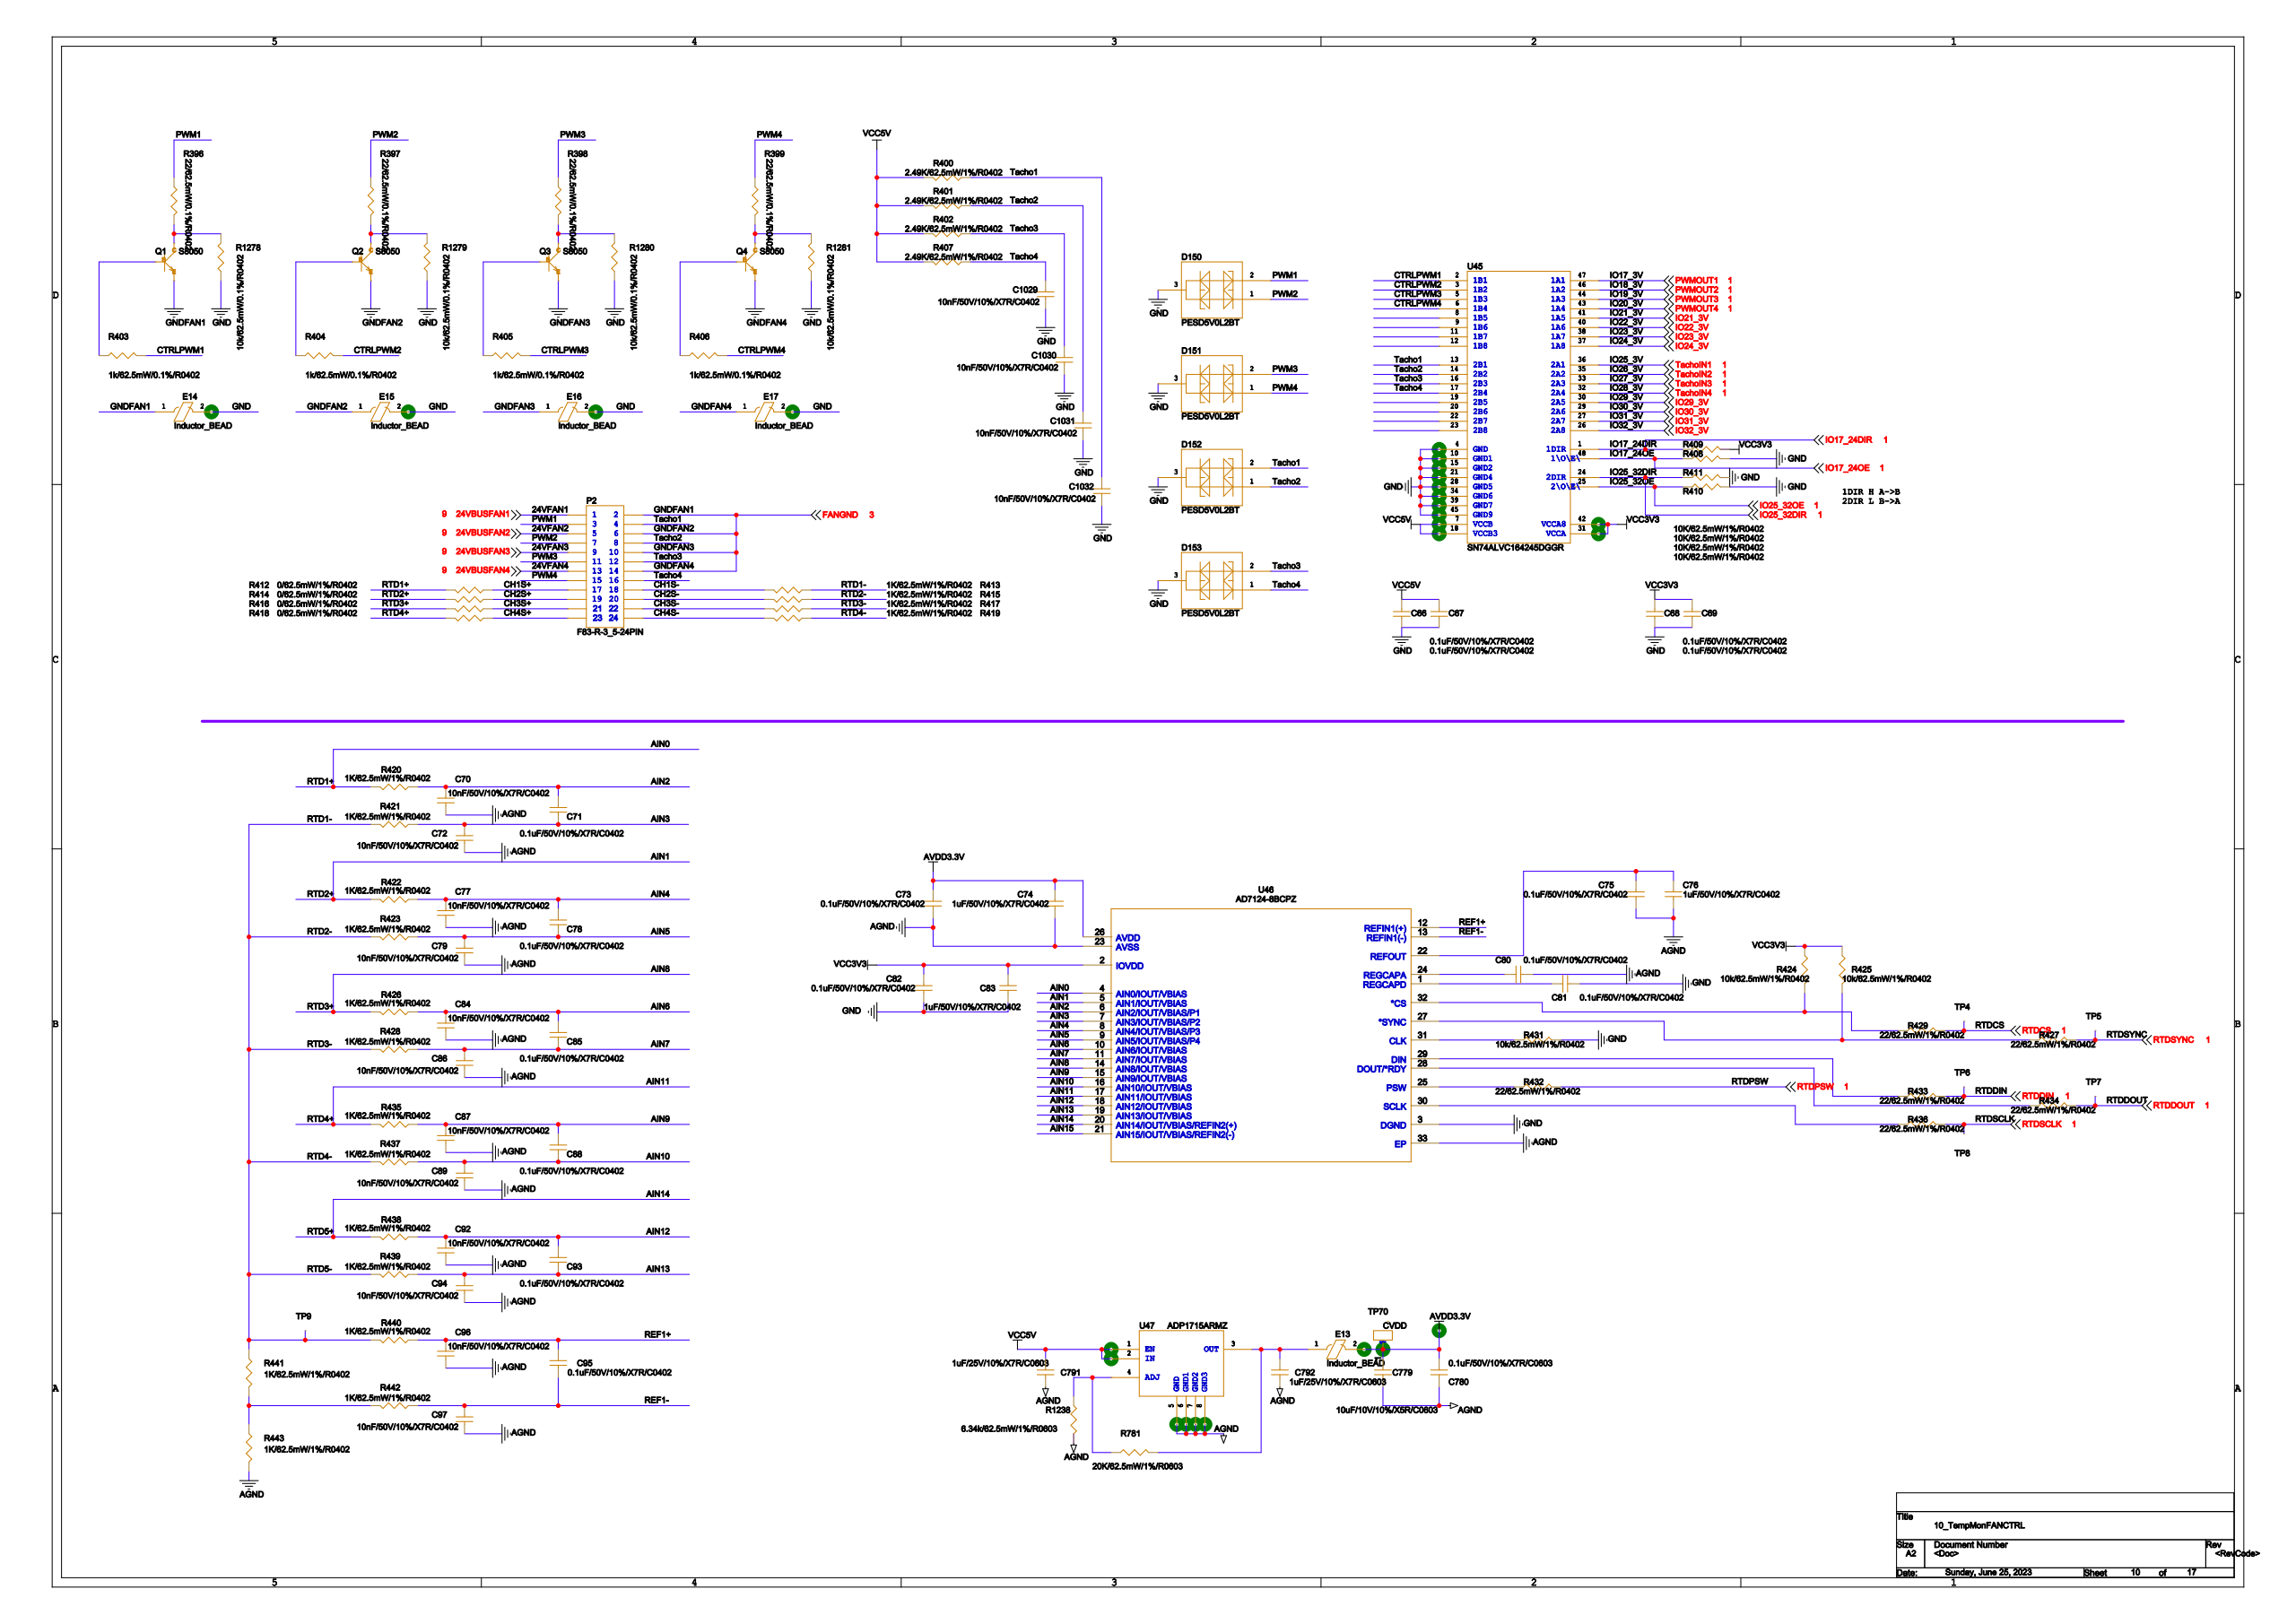Circuit board | Cadence Allegro | 2002 parts | 1538 nets | one sheet of the schematic
Parts on this sheet (reference | value | footprint):
C66 | 0.1uF/50V/10%/X7R/C0402 | 0402
C67 | 0.1uF/50V/10%/X7R/C0402 | 0402
C68 | 0.1uF/50V/10%/X7R/C0402 | 0402
C69 | 0.1uF/50V/10%/X7R/C0402 | 0402
C70 | 10nF/50V/10%/X7R/C0402 | 0402
C71 | 0.1uF/50V/10%/X7R/C0402 | 0402
C72 | 10nF/50V/10%/X7R/C0402 | 0402
C73 | 0.1uF/50V/10%/X7R/C0402 | 0402
C74 | 1uF/50V/10%/X7R/C0402 | 0402
C75 | 0.1uF/50V/10%/X7R/C0402 | 0402
C76 | 1uF/50V/10%/X7R/C0402 | 0402
C77 | 10nF/50V/10%/X7R/C0402 | 0402
C78 | 0.1uF/50V/10%/X7R/C0402 | 0402
C79 | 10nF/50V/10%/X7R/C0402 | 0402
C80 | 0.1uF/50V/10%/X7R/C0402 | 0402
C81 | 0.1uF/50V/10%/X7R/C0402 | 0402
C82 | 0.1uF/50V/10%/X7R/C0402 | 0402
C83 | 1uF/50V/10%/X7R/C0402 | 0402
C84 | 10nF/50V/10%/X7R/C0402 | 0402
C85 | 0.1uF/50V/10%/X7R/C0402 | 0402
C86 | 10nF/50V/10%/X7R/C0402 | 0402
C87 | 10nF/50V/10%/X7R/C0402 | 0402
C88 | 0.1uF/50V/10%/X7R/C0402 | 0402
C89 | 10nF/50V/10%/X7R/C0402 | 0402
C92 | 10nF/50V/10%/X7R/C0402 | 0402
C93 | 0.1uF/50V/10%/X7R/C0402 | 0402
C94 | 10nF/50V/10%/X7R/C0402 | 0402
C95 | 0.1uF/50V/10%/X7R/C0402 | 0402
C96 | 10nF/50V/10%/X7R/C0402 | 0402
C97 | 10nF/50V/10%/X7R/C0402 | 0402
C779 | 10uF/10V/10%/X5R/C0603 | 0603C
C780 | 0.1uF/50V/10%/X7R/C0603 | 0603C
C791 | 1uF/25V/10%/X7R/C0603 | 0603C
C792 | 1uF/25V/10%/X7R/C0603 | 0603C
C1029 | 10nF/50V/10%/X7R/C0402 | 0402
C1030 | 10nF/50V/10%/X7R/C0402 | 0402
C1031 | 10nF/50V/10%/X7R/C0402 | 0402
C1032 | 10nF/50V/10%/X7R/C0402 | 0402
D150 | PESD5V0L2BT | SOT23
D151 | PESD5V0L2BT | SOT23
D152 | PESD5V0L2BT | SOT23
D153 | PESD5V0L2BT | SOT23
E13 | Inductor_BEAD | 0603R
E14 | Inductor_BEAD | 0603R
E15 | Inductor_BEAD | 0603R
E16 | Inductor_BEAD | 0603R
E17 | Inductor_BEAD | 0603R
P2 | F83-R-3_5-24PIN | F83-R-3_5-24PIN
Q1 | S8050 | SOT-23
Q2 | S8050 | SOT-23
Q3 | S8050 | SOT-23
Q4 | S8050 | SOT-23
R396 | 22/62.5mW/0.1%/R0402 | 0402
R397 | 22/62.5mW/0.1%/R0402 | 0402
R398 | 22/62.5mW/0.1%/R0402 | 0402
R399 | 22/62.5mW/0.1%/R0402 | 0402
R400 | 2.49k/62.5mW/1%/R0402 | 0402
R401 | 2.49k/62.5mW/1%/R0402 | 0402
R402 | 2.49k/62.5mW/1%/R0402 | 0402
R403 | 1k/62.5mW/0.1%/R0402 | 0402
R404 | 1k/62.5mW/0.1%/R0402 | 0402
R405 | 1k/62.5mW/0.1%/R0402 | 0402
R406 | 1k/62.5mW/0.1%/R0402 | 0402
R407 | 2.49k/62.5mW/1%/R0402 | 0402
R408 | 10K/62.5mW/1%/R0402 | 0402
R409 | 10K/62.5mW/1%/R0402 | 0402
R410 | 10K/62.5mW/1%/R0402 | 0402
R411 | 10K/62.5mW/1%/R0402 | 0402
R412 | 0/62.5mW/1%/R0402 | 0402
R413 | 1K/62.5mW/1%/R0402 | 0402
R414 | 0/62.5mW/1%/R0402 | 0402
R415 | 1K/62.5mW/1%/R0402 | 0402
R416 | 0/62.5mW/1%/R0402 | 0402
R417 | 1K/62.5mW/1%/R0402 | 0402
R418 | 0/62.5mW/1%/R0402 | 0402
R419 | 1K/62.5mW/1%/R0402 | 0402
R420 | 1K/62.5mW/1%/R0402 | 0402
R421 | 1K/62.5mW/1%/R0402 | 0402
R422 | 1K/62.5mW/1%/R0402 | 0402
R423 | 1K/62.5mW/1%/R0402 | 0402
R424 | 10k/62.5mW/1%/R0402 | 0402
R425 | 10k/62.5mW/1%/R0402 | 0402
R426 | 1K/62.5mW/1%/R0402 | 0402
R427 | 22/62.5mW/1%/R0402 | 0402
R428 | 1K/62.5mW/1%/R0402 | 0402
R429 | 22/62.5mW/1%/R0402 | 0402
R431 | 10k/62.5mW/1%/R0402 | 0402
R432 | 22/62.5mW/1%/R0402 | 0402
R433 | 22/62.5mW/1%/R0402 | 0402
R434 | 22/62.5mW/1%/R0402 | 0402
R435 | 1K/62.5mW/1%/R0402 | 0402
R436 | 22/62.5mW/1%/R0402 | 0402
R437 | 1K/62.5mW/1%/R0402 | 0402
R438 | 1K/62.5mW/1%/R0402 | 0402
R439 | 1K/62.5mW/1%/R0402 | 0402
R440 | 1K/62.5mW/1%/R0402 | 0402
R441 | 1K/62.5mW/1%/R0402 | 0402
R442 | 1K/62.5mW/1%/R0402 | 0402
R443 | 1K/62.5mW/1%/R0402 | 0402
R781 | 20K/62.5mW/1%/R0603 | 0603R
R1238 | 6.34k/62.5mW/1%/R0603 | 0603R
R1278 | 10k/62.5mW/0.1%/R0402 | 0402
R1279 | 10k/62.5mW/0.1%/R0402 | 0402
R1280 | 10k/62.5mW/0.1%/R0402 | 0402
R1281 | 10k/62.5mW/0.1%/R0402 | 0402
TP4 | TEST POINT A | TEST_12MM
TP5 | TEST POINT A | TEST_12MM
TP6 | TEST POINT A | TEST_12MM
TP7 | TEST POINT A | TEST_12MM
TP8 | TEST POINT A | TEST_12MM
TP9 | TEST POINT A | TEST_12MM
TP70 | CVDD | D0_6
U45 | SN74ALVC164245DGGR | TSSOP-48
U46 | Value | CP_32_12_ADI
U47 | ADP1715ARMZ | MSOP8
Nets of these parts (net: part-pin ...):
3.3V: C68-2 C69-2 C82-1 C83-1 R409-1 R424-1 R425-1 U45-31 U45-42 U46-2
AGND: C66-1 C67-1 C68-1 C69-1 C70-2 C72-2 C73-2 C74-2 C75-2 C76-2 C77-2 C79-2 C80-2 C81-2 C82-2 C83-2 C84-2 C86-2 C87-2 C89-2 C92-2 C94-2 C96-2 C97-2 C779-2 C780-2 C791-2 C792-2 C1029-2 C1030-2 C1031-2 C1032-2 D150-3 D151-3 D152-3 D153-3 E14-2 E15-2 E16-2 E17-2 R408-1 R410-1 R411-1 R431-2 R443-2 R1238-1 R1278-1 R1279-1 R1280-1 R1281-1 U47-5 U47-6 U47-7 U47-8 U45-4 U45-10 U45-15 U45-21 U45-28 U45-34 U45-39 U45-45 U46-3 U46-23 U46-33
RTDCS: R429-2 TP4-1
RTDSCLK: R436-2 TP8-1
RTDDIN: R433-2 TP6-1
RTDDOUT: R434-2 TP7-1
RTDSYNC: R427-2 TP5-1
RTDPSW: R432-2
IO25_32DIR: R411-2 U45-24
VCC5V: C66-2 C67-2 C791-1 R400-2 R401-2 R402-2 R407-2 U47-1 U47-2 U45-7 U45-18
IO17_24OE: R408-2 U45-48
PWMOUT1: U45-47
PWMOUT2: U45-46
PWMOUT3: U45-44
PWMOUT4: U45-43
IO25_32OE: R410-2 U45-25
IO17_24DIR: R409-2 U45-1
FANGND: E14-1 E15-1 E16-1 E17-1 Q1-2 Q2-2 Q3-2 Q4-2 P2-2 P2-6 P2-10 P2-14
N24638415: Q1-3 R396-2 R1278-2
N24638411: Q2-3 R397-2 R1279-2
N24638407: Q3-3 R398-2 R1280-2
N24638403: Q4-3 R399-2 R1281-2
N24638500: Q1-1 R403-1
CTRLPWM1: R403-2 U45-2
N24638514: Q2-1 R404-1
CTRLPWM2: R404-2 U45-3
N24638545: Q3-1 R405-1
CTRLPWM3: R405-2 U45-5
N24638565: Q4-1 R406-1
CTRLPWM4: R406-2 U45-6
TACHO1: C1032-1 D152-2 R400-1 P2-4 U45-13
TACHO2: C1031-1 D152-1 R401-1 P2-8 U45-14
TACHO3: C1030-1 D153-2 R402-1 P2-12 U45-16
TACHO4: C1029-1 D153-1 R407-1 P2-16 U45-17
24VBUSFAN1: P2-1
PWM3: D151-2 R398-1 P2-11
24VBUSFAN4: P2-13
PWM4: D151-1 R399-1 P2-15
CH1S+: R412-1 P2-17
CH1S-: R413-2 P2-18
CH2S+: R414-1 P2-19
CH2S-: R415-2 P2-20
CH3S+: R416-1 P2-21
CH3S-: R417-2 P2-22
CH4S+: R418-1 P2-23
CH4S-: R419-2 P2-24
PWM1: D150-2 R396-1 P2-3
24VBUSFAN2: P2-5
PWM2: D150-1 R397-1 P2-7
24VBUSFAN3: P2-9
AVDD3.3V: C73-1 C74-1 C779-1 C780-1 E13-2 TP70-1 U46-26
N23528814: C792-1 E13-1 R781-1 U47-3
N23528786: R781-2 R1238-2 U47-4
AIN2: C70-1 C71-1 R420-1 U46-6
AIN3: C71-2 C72-1 R421-1 U46-7
N23186471: C75-1 C76-1 U46-22
AIN4: C77-1 C78-1 R422-1 U46-8
AIN5: C78-2 C79-1 R423-1 U46-9
N23186180: C80-1 U46-24
N23186182: C81-1 U46-1
AIN6: C84-1 C85-1 R426-1 U46-10
AIN7: C85-2 C86-1 R428-1 U46-11
AIN9: C87-1 C88-1 R435-1 U46-15
AIN10: C88-2 C89-1 R437-1 U46-16
AIN12: C92-1 C93-1 R438-1 U46-18
AIN13: C93-2 C94-1 R439-1 U46-19
REF1+: C95-1 C96-1 R440-1 U46-12
REF1-: C95-2 C97-1 R442-1 U46-13
RTD1-: R413-1 R415-1 R417-1 R419-1 R421-2 R423-2 R428-2 R437-2 R439-2 R440-2 R441-1 TP9-1
AIN0: R412-2 R420-2 U46-4
AIN1: R414-2 R422-2 U46-5
AIN8: R416-2 R426-2 U46-14
AIN11: R418-2 R435-2 U46-17
AIN14: R438-2 U46-20
N23184433: R441-2 R442-2 R443-1
N23186319: R424-2 R429-1 U46-32
N23186325: R425-2 R427-1 U46-27
N23186239: R431-1 U46-31
N23186243: R432-1 U46-25
N23186381: R433-1 U46-29
N23186383: R434-1 U46-28
N23186389: R436-1 U46-30
IO21_3V: U45-41
IO22_3V: U45-40
IO23_3V: U45-38
IO24_3V: U45-37
IO29_3V: U45-30
IO30_3V: U45-29
IO31_3V: U45-27
IO32_3V: U45-26
AIN15: U46-21